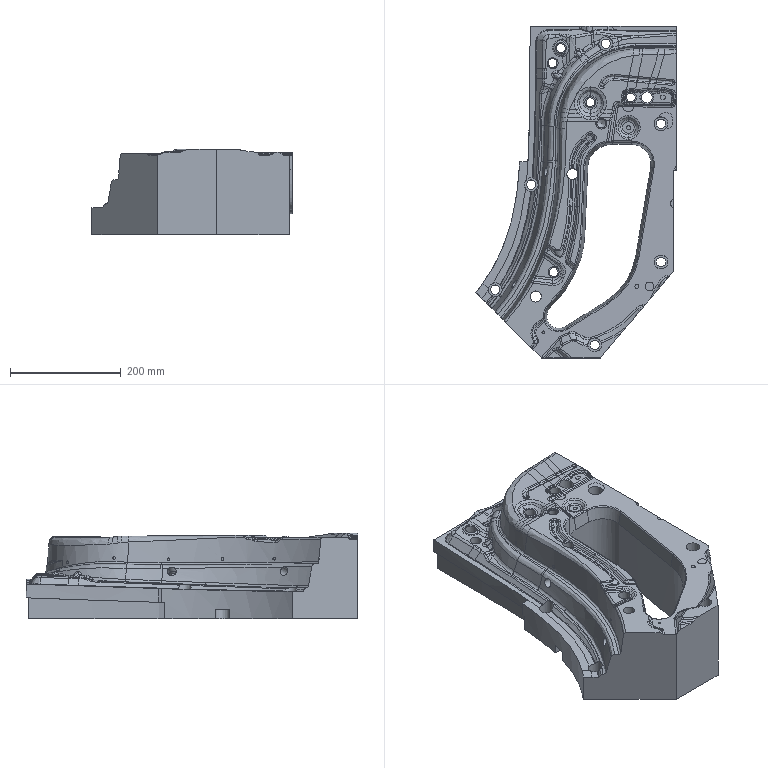Part | NX | features solid 2 | 1 solid | 647 faces | box 362.205 x 600.69 x 154.902 mm | volume 13100407 mm3 | spline 566 | cylinder 43 | plane 37 | cone 1 | commonest cylinder face diameters 25 x12 20 x9 16 x8 17 x6 23 x5 13 x2